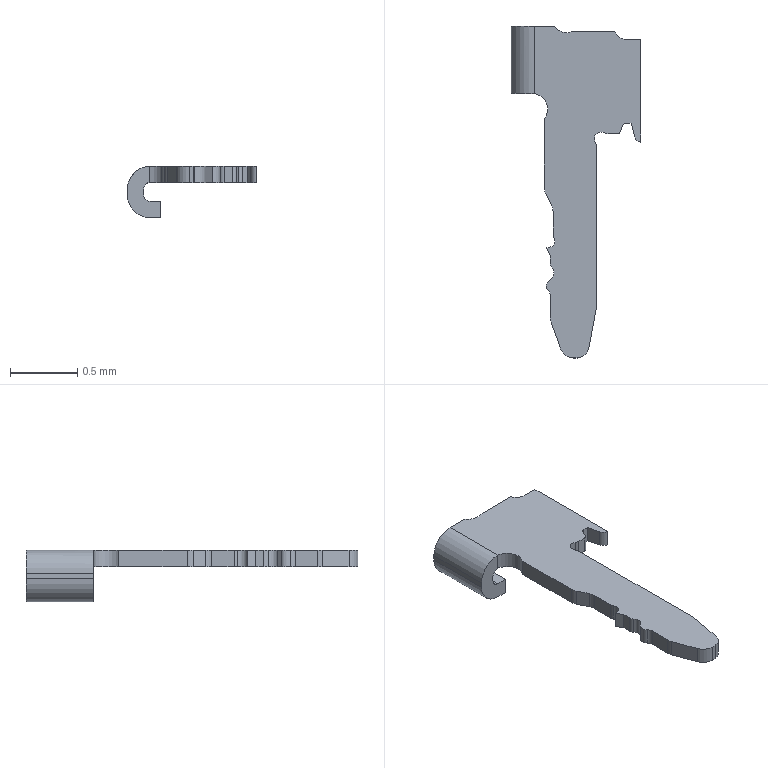Part | Creo | 1 solid | 53 faces | box 0.96 x 2.46 x 0.38 mm | volume 0.1621 mm3 | plane 29 | cylinder 24 | commonest cylinder face diameters 0.1 x12 0.2 x7 0.06 x2 0.34 x2 0.232 x1